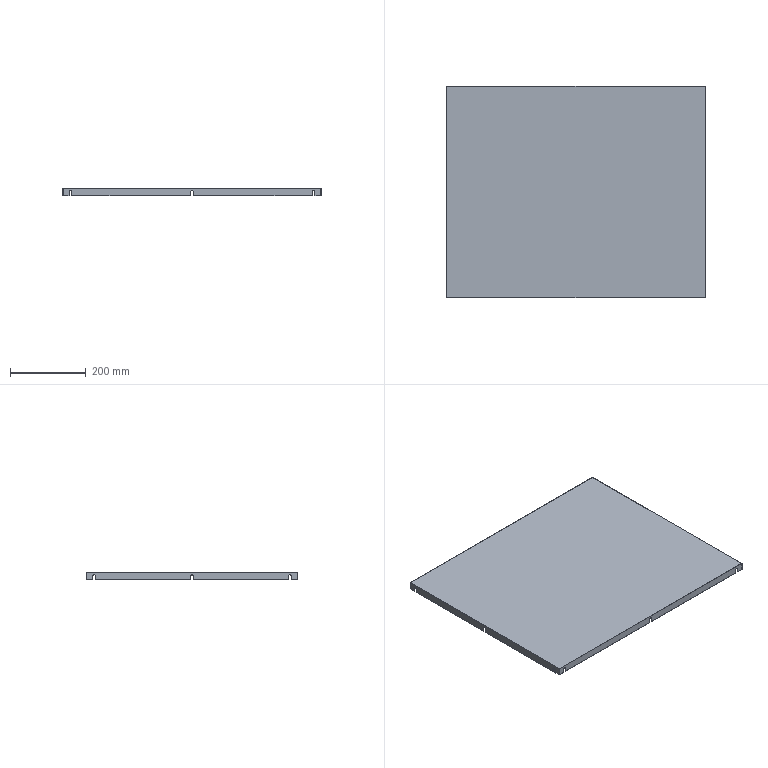Part | STEP file | 1 solid | 64 faces | box 683 x 558 x 20 mm | volume 427125 mm3 | plane 46 | cylinder 18 | commonest cylinder face diameters 7 x18